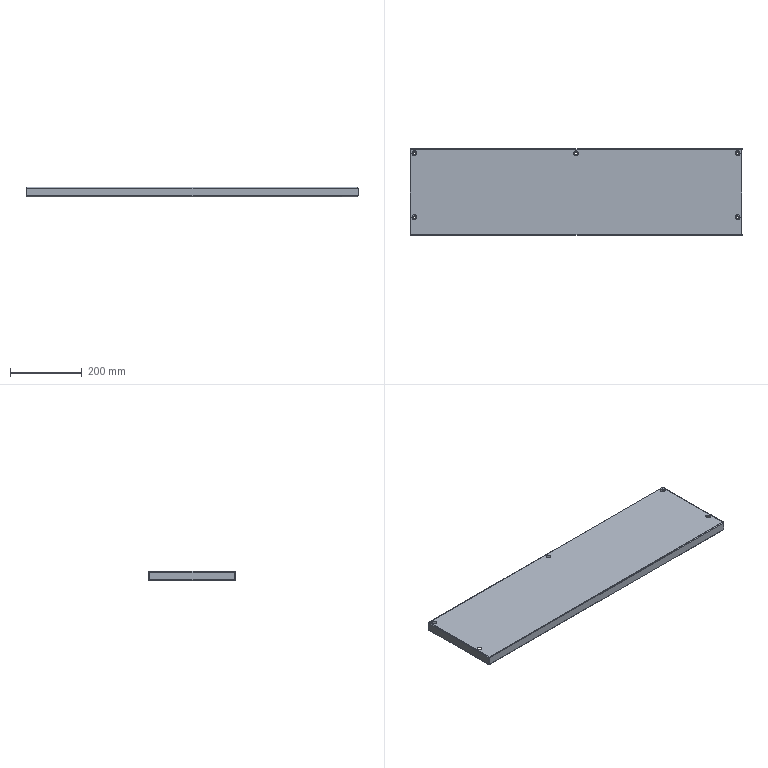Part | STEP file | Rear Panel Middle | 1 solid | 121 faces | box 923 x 240 x 26 mm | volume 474595 mm3 | plane 66 | cylinder 39 | spline 16 | commonest cylinder face diameters 7 x13 13 x10 1 x8 4 x8